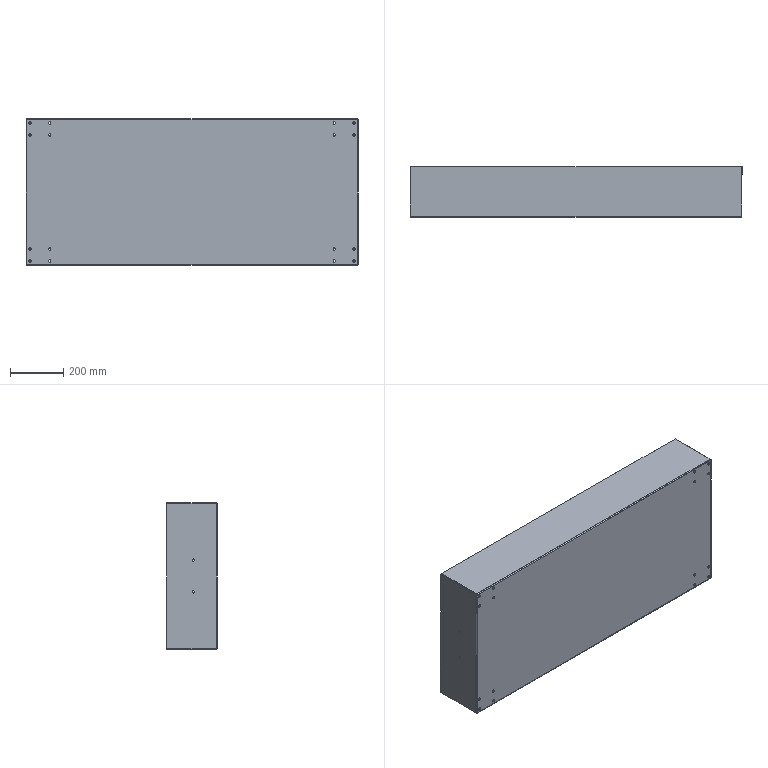Part | SolidWorks | features HoleWzd 3, MirrorPattern 2, EdgeFlange 1, FlatPattern 1, LPattern 1, SMBaseFlange 1, SheetMetal 1, WeldmentFeature 1 | 1 solid | 82 faces | box 1250 x 190 x 550 mm | volume 4050815 mm3 | cylinder 52 | plane 22 | spline 8 | commonest cylinder face diameters 9 x44 1.473 x4 7.473 x4